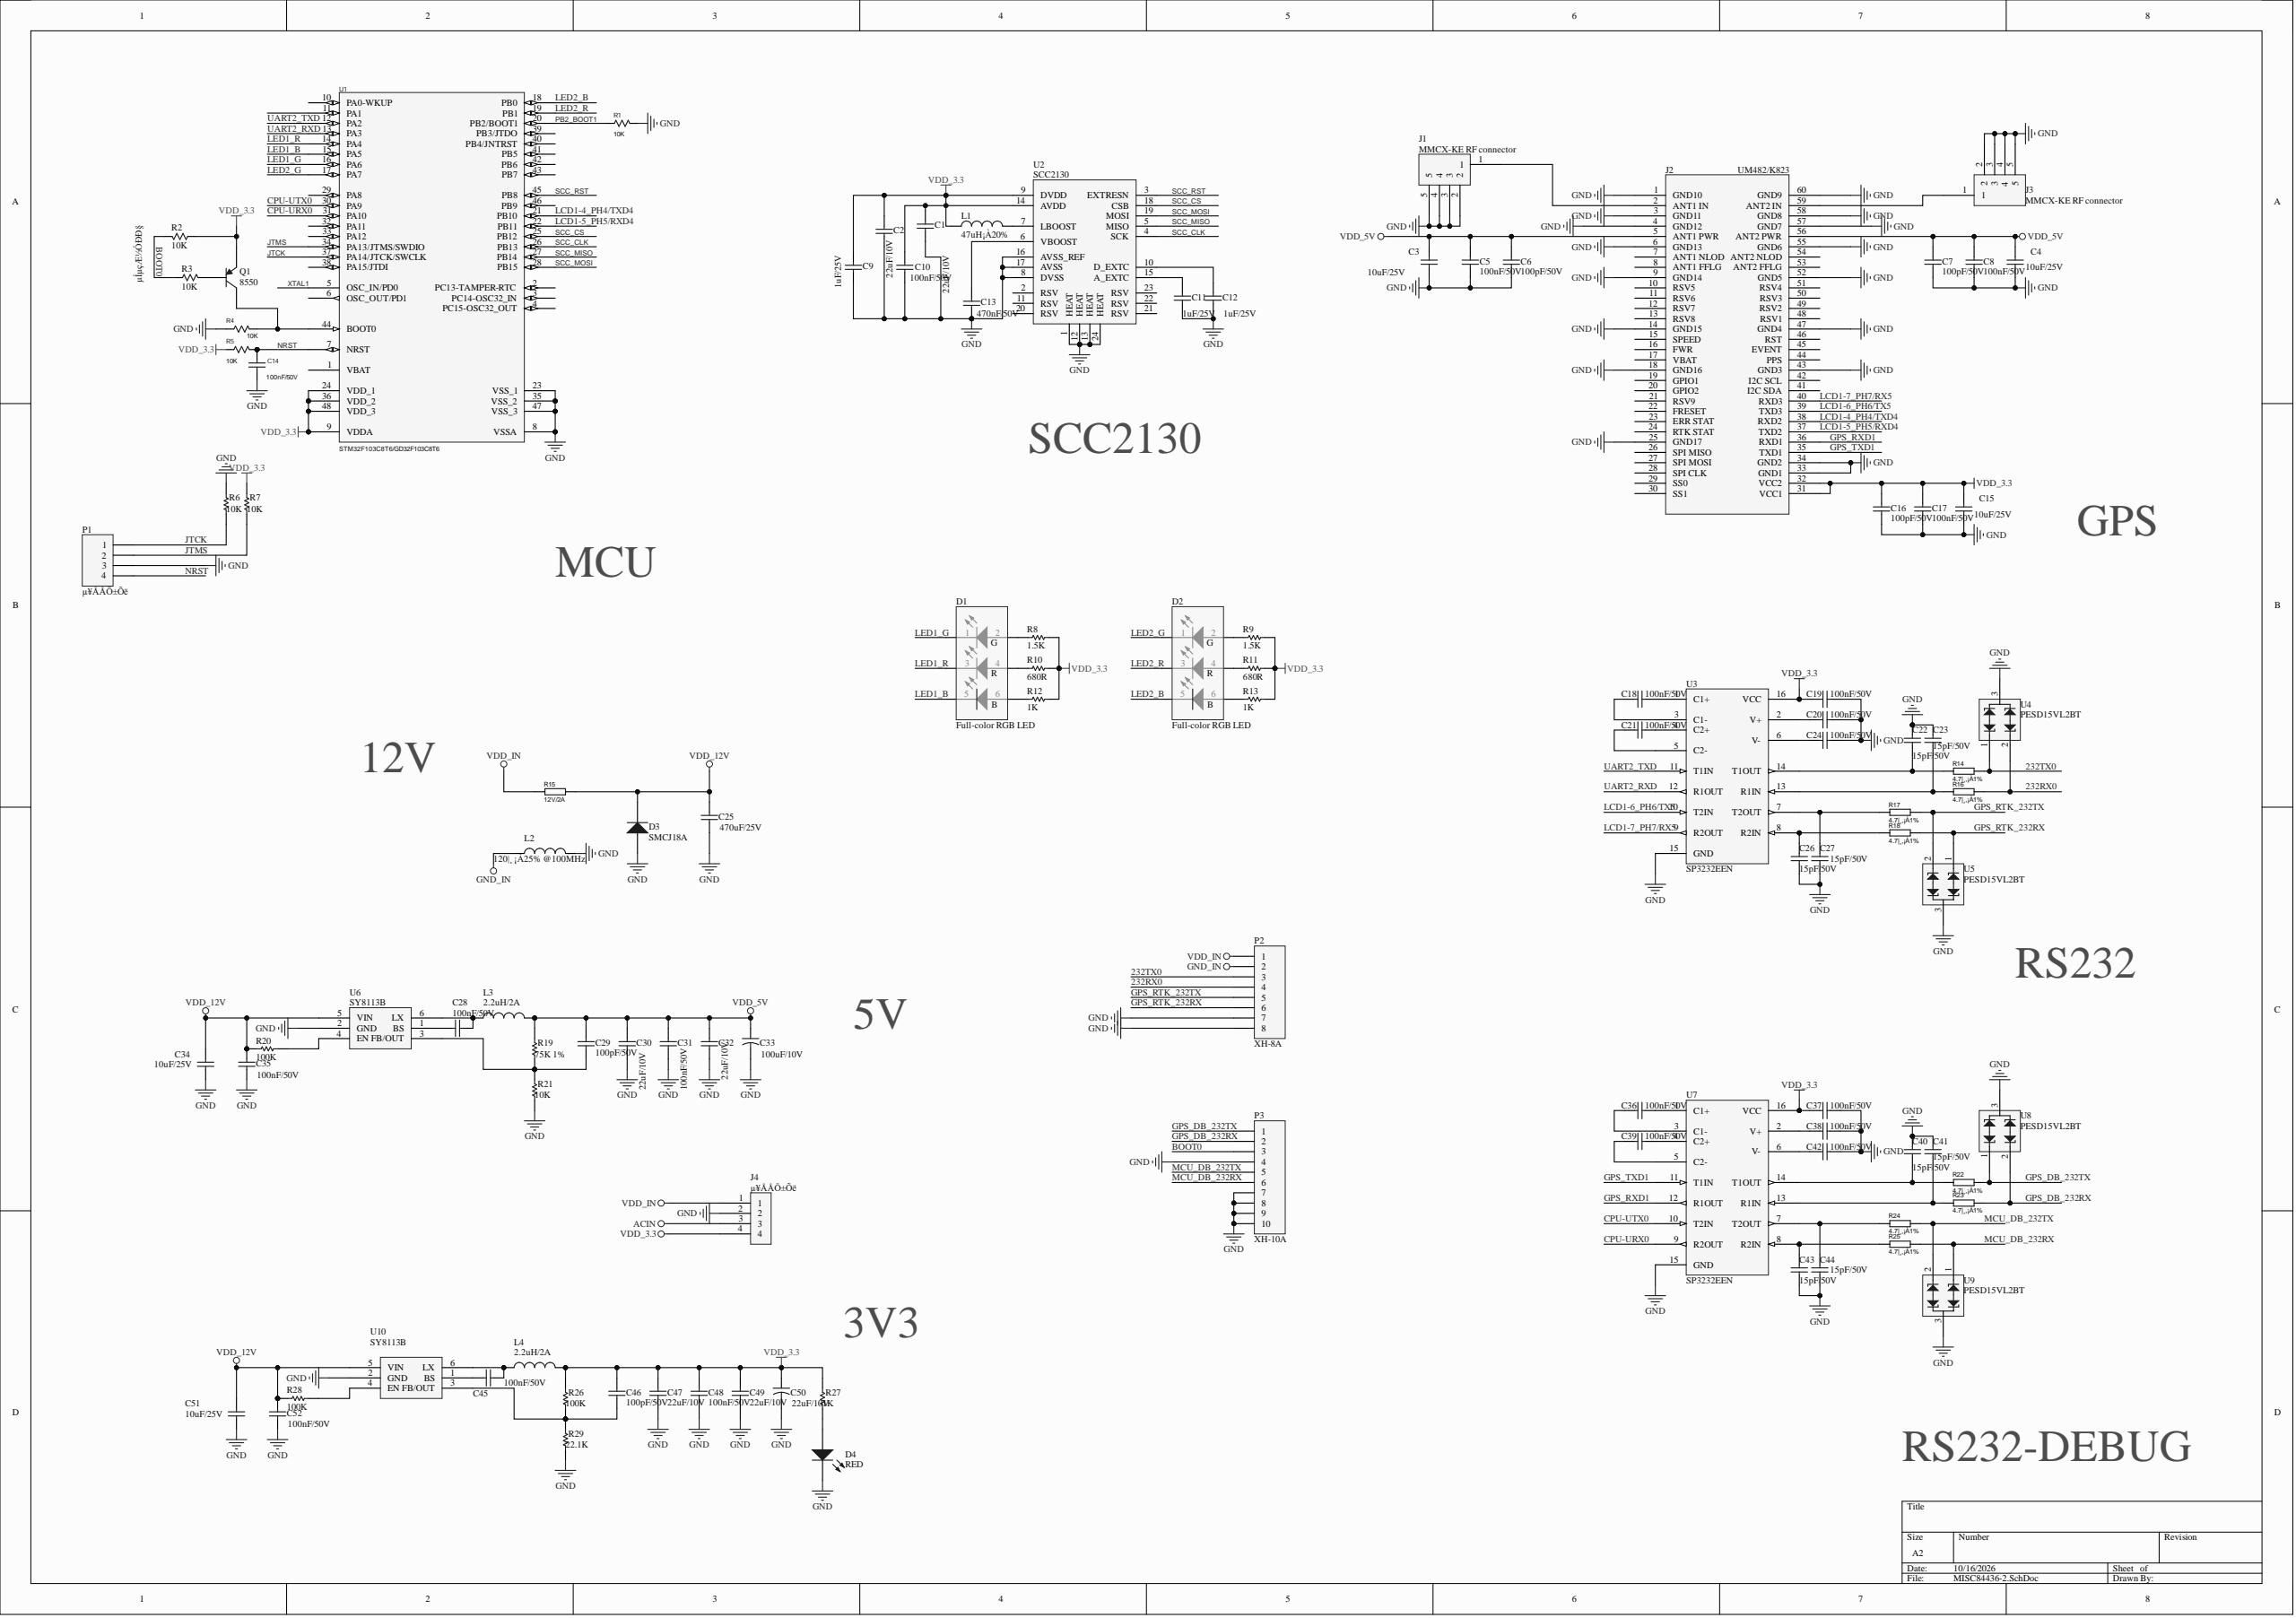Circuit board | Altium Designer | 107 parts | 83 nets
Bill of materials:
Comment,Description,Designator,Footprint,LibRef,Quantity
"22uF/10V","SMD ceramic capacitor,X5R, Capacitor","C1, C2, C30, C32, C47, C49, C50","C0805","Cap, Cap2","7"
"10uF/25V","SMD ceramic capacitor,X7R, SMD ceramic capacitor,MLCC, Capacitor","C3, C4, C15, C34, C51","C0805","Cap","5"
"100nF/50V","表贴陶瓷电容, SMD ceramic capacitor,X7R, Capacitor, SMD capacitor,X7R","C5, C8, C10, C14, C17, C18, C19, C20, C21, C24, C28, C31, C35, C36, C37, C38, C39, C42, C45, C48, C52","0603","Cap","21"
"100pF/50V","表贴陶瓷电容, Capacitor","C6, C7, C16, C29, C46","0603","Cap","5"
"1uF/25V","SMD ceramic capacitor,X7R","C9, C11, C12","0603","Cap","3"
"470nF/50V","SMD ceramic capacitor,X7R","C13","0603","Cap","1"
"15pF/50V","SMD capacitor,X7R","C22, C23, C26, C27, C40, C41, C43, C44","0603","Cap","8"
"470uF/25V","470|ÌF,25V,§¶8¡Á11.5mm,RoHS","C25","CAP-TH_BD8.0-P3.50-D1.0-FD","Cap","1"
"100uF/10V","100|ÌF,10V,§¶5¡Á7mm,RoHS","C33","CAP-TH_BD5.0-P2.00-D0.8-FD","Cap2","1"
"Full-color RGB LED","19-337C/RSBHGHC-M03/2T,EVERLIGHT (Taiwan)","D1, D2","RGB","LED1_3","2"
"SMCJ18A","TVS diode","D3","SMC_L6.9-W5.9-LS7.9-RD","Diode","1"
"RED","Red high-brightness LED","D4","LED_0805","LED1","1"
"MMCX-KE RF connector","","J1, J3","MMCX-TH_ZC11.801KK","CIRCLE","2"
"UM482/K823","高精度卫星接收机","J2","UM482/K823","UM482","1"
"单排直针","Single-row straight header,4P,2.54mm","J4, P1","HDR1X4","2.54, Header 4","2"
"47uH¡À20%","表贴电感","L1","1210","Inductor","1"
"120|¸ ¡À25% @100MHz","磁珠","L2","0603","Inductor","1"
"2.2uH/2A","SMD power inductor,cjiang,FNR4026S2R2MT","L3, L4","IND-SMD_L4.0-W4.0","Inductor","2"
"XH-8A","8P,pitch 2.5mm,through-hole,BOOMELE","P2","CONN-TH_XH-8A","Header 8","1"
"XH-10A","10P,pitch 2.5mm,through-hole,BOOMELE","P3","CONN-TH_10P-P2.50_XH-10A","Header 10","1"
"8550","PNP Bipolar Transistor","Q1","SOT-23-SS8550","PNP","1"
"10K","表贴电阻, 标贴电阻","R1, R2, R3, R4, R5, R6, R7, R21","0603","Res, Res1","8"
"1.5K","表贴电阻","R8, R9","0603","Res1","2"
"680R","表贴电阻","R10, R11","0603","Res1","2"
"1K","表贴电阻","R12, R13, R27","0603","Res1","3"
"4.7|¸,¡À1%","表贴电阻","R14, R16, R17, R18, R22, R23, R24, R25","0603","RES","8"
"12V/2A","自恢复保险丝","R15","1210","RES","1"
"75K 1%","表贴电阻","R19","0603","Res1","1"
"100K","表贴电阻","R20, R26, R28","0603","Res1","3"
"22.1K","表贴电阻","R29","0603","Res1","1"
"STM32F103C8T6/GD32F103C8T6","STM32 ARM-based 32-bit MCU with ST/GD GigaDevice","U1","LQFP-48_L7.0-W7.0-P0.50-LS9.0-BL","STM32F103C8T6","1"
"SCC2130","MEMS digital gyroscope","U2","SCC2130D","SCC2130","1"
"SP3232EEN","","U3, U7","SOP16-6.6","SP202ECT","2"
"PESD15VL2BT","","U4, U5, U8, U9","SOT-23","PESD12VL2BT","4"
"SY8113B","","U6, U10","TSOT-23-6_L2.9-W1.6-P0.95-LS2.8-BR","SY8113B","2"
Netlist (Protel format):
[
C1
C0805
22uF/10V



]
[
C2
C0805
22uF/10V



]
[
C3
C0805
10uF/25V



]
[
C4
C0805
10uF/25V



]
[
C5
0603
100nF/50V



]
[
C6
0603
100pF/50V



]
[
C7
0603
100pF/50V



]
[
C8
0603
100nF/50V



]
[
C9
0603
1uF/25V



]
[
C10
0603
100nF/50V



]
[
C11
0603
1uF/25V



]
[
C12
0603
1uF/25V



]
[
C13
0603
470nF/50V



]
[
C14
0603
100nF/50V



]
[
C15
C0805
10uF/25V



]
[
C16
0603
100pF/50V



]
[
C17
0603
100nF/50V



]
[
C18
0603
100nF/50V



]
[
C19
0603
100nF/50V



]
[
C20
0603
100nF/50V



]
[
C21
0603
100nF/50V



]
[
C22
0603
15pF/50V



]
[
C23
0603
15pF/50V



]
[
C24
0603
100nF/50V



]
[
C25
CAP-TH_BD8.0-P3.50-D1.0-FD
470uF/25V



]
[
C26
0603
15pF/50V



]
[
C27
0603
15pF/50V



]
[
C28
0603
100nF/50V



]
[
C29
0603
100pF/50V



]
[
C30
C0805
22uF/10V



]
[
C31
0603
100nF/50V



]
[
C32
C0805
22uF/10V



]
[
C33
CAP-TH_BD5.0-P2.00-D0.8-FD
100uF/10V



]
[
C34
C0805
10uF/25V



]
[
C35
0603
100nF/50V



]
[
C36
0603
100nF/50V



]
[
C37
0603
100nF/50V



]
[
C38
0603
100nF/50V



]
[
C39
0603
100nF/50V



]
[
C40
0603
15pF/50V



]
[
C41
0603
15pF/50V



]
[
C42
0603
100nF/50V



]
[
C43
0603
15pF/50V



]
[
C44
0603
15pF/50V



]
[
C45
0603
100nF/50V



]
[
C46
0603
100pF/50V



]
[
C47
C0805
22uF/10V



]
[
C48
0603
100nF/50V



]
[
C49
C0805
22uF/10V



]
[
C50
C0805
22uF/10V



]
[
C51
C0805
10uF/25V



]
[
C52
0603
100nF/50V



]
[
D1
RGB
Full-color RGB LED



]
[
D2
RGB
Full-color RGB LED



]
[
D3
SMC_L6.9-W5.9-LS7.9-RD
SMCJ18A



]
[
D4
LED_0805
RED



]
[
J1
MMCX-TH_ZC11.801KK
MMCX-KE RF connector



]
[
J2
UM482/K823
UM482/K823



]
[
J3
MMCX-TH_ZC11.801KK
MMCX-KE RF connector



]
[
J4
HDR1X4
单排直针



]
[
L1
1210
47uH¡À20%



]
[
L2
0603
120|¸ ¡À25% @100MHz



]
[
L3
IND-SMD_L4.0-W4.0
2.2uH/2A



]
[
L4
IND-SMD_L4.0-W4.0
2.2uH/2A



]
[
P1
HDR1X4
单排直针



]
[
P2
CONN-TH_XH-8A
XH-8A



]
[
P3
CONN-TH_10P-P2.50_XH-10A
XH-10A



]
[
Q1
SOT-23-SS8550
8550



]
[
R1
0603
10K



]
[
R2
0603
10K



]
[
R3
0603
10K



]
[
R4
0603
10K



]
[
R5
0603
10K



]
[
R6
0603
10K



]
[
R7
0603
10K



]
[
R8
0603
1.5K



]
[
R9
0603
1.5K



]
[
R10
0603
680R



]
[
R11
0603
680R



]
[
R12
0603
1K



]
[
R13
0603
1K



]
[
R14
0603
4.7|¸,¡À1%



]
[
R15
1210
12V/2A



]
[
R16
0603
4.7|¸,¡À1%



]
[
R17
0603
4.7|¸,¡À1%



]
[
R18
0603
4.7|¸,¡À1%



]
[
R19
0603
75K 1%



]
[
R20
0603
100K



]
[
R21
0603
10K



]
[
R22
0603
4.7|¸,¡À1%



]
[
R23
0603
4.7|¸,¡À1%



]
[
R24
0603
4.7|¸,¡À1%



]
[
R25
0603
4.7|¸,¡À1%



]
[
R26
0603
100K



]
[
R27
0603
1K



]
[
R28
0603
100K



]
[
R29
0603
22.1K



]
[
U1
LQFP-48_L7.0-W7.0-P0.50-LS9.0-BL
STM32F103C8T6/GD32F103C8T6



]
[
U2
SCC2130D
SCC2130



]
[
U3
SOP16-6.6
SP3232EEN



]
[
U4
SOT-23
PESD15VL2BT



]
[
U5
SOT-23
PESD15VL2BT



]
[
U6
TSOT-23-6_L2.9-W1.6-P0.95-LS2.8-BR
SY8113B



]
[
U7
SOP16-6.6
SP3232EEN



]
[
U8
SOT-23
PESD15VL2BT



]
[
U9
SOT-23
PESD15VL2BT



]
[
U10
TSOT-23-6_L2.9-W1.6-P0.95-LS2.8-BR
SY8113B



]
(
VDD_IN
J4-1
P2-1
R15-2
)
(
VDD_12V
C25-1
C34-2
C35-2
C51-2
C52-2
D3-2
R15-1
R20-2
R28-2
U6-5
U10-5
)
(
VDD_5V
C3-2
C4-2
C5-1
C6-1
C7-2
C8-2
C29-1
C30-1
C31-1
C32-1
C33-1
J2-5
J2-56
L3-2
R19-2
)
(
VDD_3.3
C1-1
C2-1
C9-1
C10-1
C15-2
C16-2
C17-2
C19-1
C37-1
C46-1
C47-1
C48-1
C49-1
C50-1
J2-31
J2-32
J4-4
L1-1
L4-2
Q1-2
R2-2
R5-2
R7-2
R8-1
R9-1
R10-1
R11-1
R12-1
R13-1
R26-2
R27-2
U1-9
U1-24
U1-36
U1-48
U2-9
U2-14
U3-16
U7-16
)
(
UART2_TXD
U1-12
U3-11
)
(
UART2_RXD
U1-13
U3-12
)
(
SCC_RST
U1-45
U2-3
)
(
SCC_MOSI
U1-28
U2-19
)
(
SCC_MISO
U1-27
U2-5
)
(
SCC_CS
U1-25
U2-18
)
(
SCC_CLK
U1-26
U2-4
)
(
PB2_BOOT1
R1-2
U1-20
)
(
NRST
C14-2
P1-4
R5-1
U1-7
)
(
NetR28_1
R28-1
U10-4
)
(
NetR20_1
R20-1
U6-4
)
(
NetQ1_3
Q1-3
R4-2
U1-44
)
(
NetQ1_1
Q1-1
R3-1
)
(
NetL1_2
L1-2
U2-7
)
(
NetJ2_59
J2-59
J3-1
)
(
NetJ1_1
J1-1
J2-2
)
(
NetD4_1
D4-1
R27-1
)
(
NetD2_6
D2-6
R13-2
)
(
NetD2_4
D2-4
R11-2
)
(
NetD2_2
D2-2
R9-2
)
(
NetD1_6
D1-6
R12-2
)
(
NetD1_4
D1-4
R10-2
)
(
NetD1_2
D1-2
R8-2
)
(
NetC46_2
C46-2
R26-1
R29-2
U10-3
)
(
NetC45_2
C45-2
U10-1
)
(
NetC45_1
C45-1
L4-1
U10-6
)
(
NetC44_1
C44-1
R24-2
U7-7
)
(
NetC43_1
C43-1
R25-2
U7-8
)
(
NetC42_1
C42-1
U7-6
)
(
NetC41_2
C41-2
R23-2
U7-13
)
(
NetC40_2
C40-2
R22-2
U7-14
)
(
NetC39_2
C39-2
U7-4
)
(
NetC39_1
C39-1
U7-5
)
(
NetC38_1
C38-1
U7-2
)
(
NetC36_2
C36-2
U7-1
)
(
NetC36_1
C36-1
U7-3
)
(
NetC29_2
C29-2
R19-1
R21-2
U6-3
)
(
NetC28_2
C28-2
U6-1
)
(
NetC28_1
C28-1
L3-1
U6-6
)
(
NetC27_1
C27-1
R17-2
U3-7
)
(
NetC26_1
C26-1
R18-2
U3-8
)
(
NetC24_1
C24-1
U3-6
)
(
NetC23_2
C23-2
R16-2
U3-13
)
(
NetC22_2
C22-2
R14-2
U3-14
)
(
NetC21_2
C21-2
U3-4
)
(
NetC21_1
C21-1
U3-5
)
(
NetC20_1
C20-1
U3-2
)
(
NetC18_2
C18-2
U3-1
)
(
NetC18_1
C18-1
U3-3
)
(
NetC13_1
C13-1
U2-6
)
(
NetC12_1
C12-1
U2-10
)
(
NetC11_1
C11-1
U2-15
)
(
MCU_DB_232TX
P3-5
R24-1
U9-2
)
(
MCU_DB_232RX
P3-6
R25-1
U9-1
)
(
LED2_R
D2-3
U1-19
)
(
LED2_G
D2-1
U1-17
)
(
LED2_B
D2-5
U1-18
)
(
LED1_R
D1-3
U1-14
)
(
LED1_G
D1-1
U1-16
)
(
LED1_B
D1-5
U1-15
)
(
LCD1-7_PH7/RX5
J2-40
U3-9
)
(
LCD1-6_PH6/TX5
J2-39
U3-10
)
(
LCD1-5_PH5/RXD4
J2-37
U1-22
)
(
LCD1-4_PH4/TXD4
J2-38
U1-21
)
(
JTMS
P1-2
R7-1
U1-34
)
(
JTCK
P1-1
R6-1
U1-37
)
(
GPS_TXD1
J2-35
U7-11
)
(
GPS_RXD1
J2-36
U7-12
)
(
GPS_RTK_232TX
P2-5
R17-1
U5-2
)
(
GPS_RTK_232RX
P2-6
R18-1
U5-1
)
(
GPS_DB_232TX
P3-1
R22-1
U8-1
)
(
GPS_DB_232RX
P3-2
R23-1
U8-2
)
(
GND_IN
L2-1
P2-2
)
(
GND
C1-2
C2-2
C3-1
C4-1
C5-2
C6-2
C7-1
C8-1
C9-2
C10-2
C11-2
C12-2
C13-2
C14-1
C15-1
C16-1
C17-1
C19-2
C20-2
C22-1
C23-1
C24-2
C25-2
C26-2
C27-2
C30-2
C31-2
C32-2
C33-2
C34-1
C35-1
C37-2
C38-2
C40-1
C41-1
C42-2
C43-2
C44-2
C47-2
C48-2
C49-2
C50-2
C51-1
C52-1
D3-1
D4-2
J1-2
J1-3
J1-4
J1-5
J2-1
J2-3
J2-4
J2-6
J2-9
J2-14
J2-18
J2-25
J2-33
J2-34
J2-43
J2-47
J2-52
J2-55
J2-57
J2-58
J2-60
J3-2
J3-3
J3-4
J3-5
J4-2
L2-2
P1-3
P2-7
P2-8
P3-4
P3-7
P3-8
P3-9
P3-10
R1-1
R4-1
R6-2
R21-1
R29-1
U1-8
U1-23
U1-35
U1-47
U2-1
U2-8
U2-12
U2-13
U2-16
U2-17
U2-24
U3-15
U4-3
U5-3
U6-2
U7-15
U8-3
U9-3
U10-2
)
(
CPU-UTX0
U1-30
U7-10
)
(
CPU-URX0
U1-31
U7-9
)
(
BOOT0
P3-3
R2-1
R3-2
)
(
232TX0
P2-3
R14-1
U4-1
)
(
232RX0
P2-4
R16-1
U4-2
)